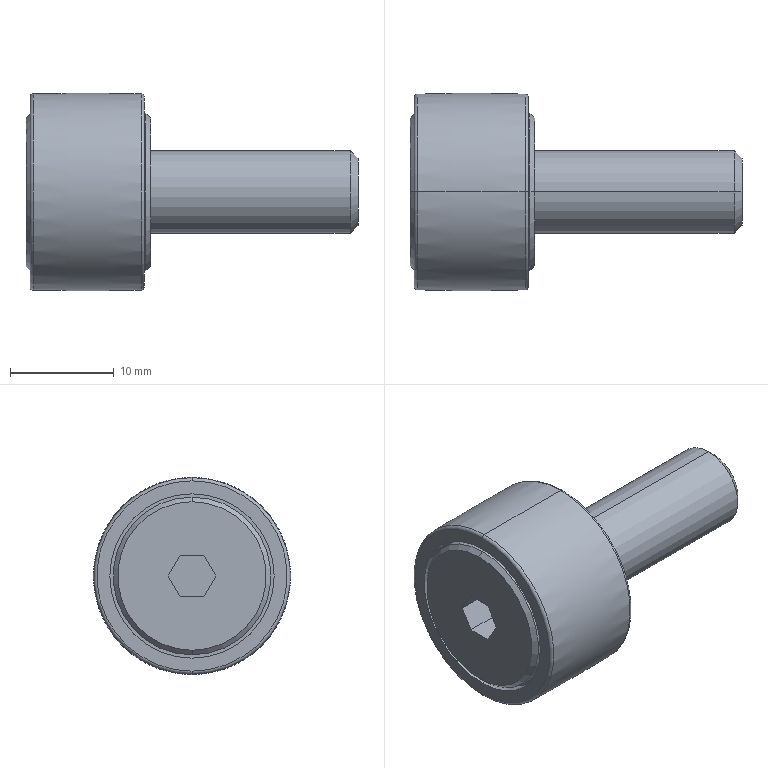Part | STEP file | CF8MUUR-A-1 | 1 solid | 36 faces | box 32 x 19 x 19 mm | volume 4191 mm3 | plane 14 | cylinder 10 | cone 6 | torus 6 | commonest cylinder face diameters 15.2 x4 15.833 x4 8 x2
STEP:
#1=CARTESIAN_POINT('',(32.,0.,-3.233));
#2=VERTEX_POINT('',#1);
#3=CARTESIAN_POINT('',(32.,0.,3.233));
#4=VERTEX_POINT('',#3);
#5=CARTESIAN_POINT('',(32.,0.,0.));
#6=DIRECTION('',(1.,0.,0.));
#7=DIRECTION('',(0.,0.,-1.));
#8=AXIS2_PLACEMENT_3D('',#5,#6,#7);
#9=CIRCLE('',#8,3.233);
#10=EDGE_CURVE('',#2,#4,#9,.T.);
#11=ORIENTED_EDGE('',*,*,#10,.F.);
#12=CARTESIAN_POINT('',(31.233,0.,-4.));
#13=VERTEX_POINT('',#12);
#14=CARTESIAN_POINT('',(31.233,0.,-4.));
#15=DIRECTION('',(-0.7071,0.,-0.7071));
#16=VECTOR('',#15,1000.);
#17=LINE('',#14,#16);
#18=EDGE_CURVE('',#2,#13,#17,.T.);
#19=ORIENTED_EDGE('',*,*,#18,.T.);
#20=CARTESIAN_POINT('',(31.233,0.,4.));
#21=VERTEX_POINT('',#20);
#22=CARTESIAN_POINT('',(31.233,0.,0.));
#23=DIRECTION('',(1.,0.,0.));
#24=DIRECTION('',(0.,0.,-1.));
#25=AXIS2_PLACEMENT_3D('',#22,#23,#24);
#26=CIRCLE('',#25,4.);
#27=EDGE_CURVE('',#13,#21,#26,.T.);
#28=ORIENTED_EDGE('',*,*,#27,.T.);
#29=CARTESIAN_POINT('',(31.233,0.,4.));
#30=DIRECTION('',(-0.7071,0.,0.7071));
#31=VECTOR('',#30,1000.);
#32=LINE('',#29,#31);
#33=EDGE_CURVE('',#4,#21,#32,.T.);
#34=ORIENTED_EDGE('',*,*,#33,.F.);
#35=EDGE_LOOP('',(#11,#19,#28,#34));
#36=FACE_OUTER_BOUND('',#35,.T.);
#37=CARTESIAN_POINT('',(31.233,0.,0.));
#38=DIRECTION('',(-1.,0.,0.));
#39=DIRECTION('',(0.,0.,1.));
#40=AXIS2_PLACEMENT_3D('',#37,#38,#39);
#41=CONICAL_SURFACE('',#40,4.,0.7854);
#42=ADVANCED_FACE('',(#36),#41,.T.);
#43=CARTESIAN_POINT('',(12.,0.,-4.));
#44=VERTEX_POINT('',#43);
#45=CARTESIAN_POINT('',(12.,0.,4.));
#46=VERTEX_POINT('',#45);
#47=CARTESIAN_POINT('',(12.,0.,0.));
#48=DIRECTION('',(1.,0.,0.));
#49=DIRECTION('',(0.,0.,-1.));
#50=AXIS2_PLACEMENT_3D('',#47,#48,#49);
#51=CIRCLE('',#50,4.);
#52=EDGE_CURVE('',#44,#46,#51,.T.);
#53=ORIENTED_EDGE('',*,*,#52,.T.);
#54=CARTESIAN_POINT('',(32.,0.,4.));
#55=DIRECTION('',(1.,0.,0.));
#56=VECTOR('',#55,1000.);
#57=LINE('',#54,#56);
#58=EDGE_CURVE('',#46,#21,#57,.T.);
#59=ORIENTED_EDGE('',*,*,#58,.T.);
#60=ORIENTED_EDGE('',*,*,#27,.F.);
#61=CARTESIAN_POINT('',(32.,0.,-4.));
#62=DIRECTION('',(1.,0.,0.));
#63=VECTOR('',#62,1000.);
#64=LINE('',#61,#63);
#65=EDGE_CURVE('',#44,#13,#64,.T.);
#66=ORIENTED_EDGE('',*,*,#65,.F.);
#67=EDGE_LOOP('',(#53,#59,#60,#66));
#68=FACE_OUTER_BOUND('',#67,.T.);
#69=CARTESIAN_POINT('',(32.,0.,0.));
#70=DIRECTION('',(1.,0.,0.));
#71=DIRECTION('',(0.,0.,-1.));
#72=AXIS2_PLACEMENT_3D('',#69,#70,#71);
#73=CYLINDRICAL_SURFACE('',#72,4.);
#74=ADVANCED_FACE('',(#68),#73,.T.);
#75=CARTESIAN_POINT('',(12.,0.,-7.16));
#76=VERTEX_POINT('',#75);
#77=CARTESIAN_POINT('',(12.,0.,7.16));
#78=VERTEX_POINT('',#77);
#79=CARTESIAN_POINT('',(12.,0.,0.));
#80=DIRECTION('',(1.,0.,0.));
#81=DIRECTION('',(0.,0.,-1.));
#82=AXIS2_PLACEMENT_3D('',#79,#80,#81);
#83=CIRCLE('',#82,7.16);
#84=EDGE_CURVE('',#76,#78,#83,.T.);
#85=ORIENTED_EDGE('',*,*,#84,.F.);
#86=CARTESIAN_POINT('',(11.56,0.,-7.6));
#87=VERTEX_POINT('',#86);
#88=CARTESIAN_POINT('',(11.56,0.,-7.6));
#89=DIRECTION('',(-0.7071,0.,-0.7071));
#90=VECTOR('',#89,1000.);
#91=LINE('',#88,#90);
#92=EDGE_CURVE('',#76,#87,#91,.T.);
#93=ORIENTED_EDGE('',*,*,#92,.T.);
#94=CARTESIAN_POINT('',(11.56,0.,7.6));
#95=VERTEX_POINT('',#94);
#96=CARTESIAN_POINT('',(11.56,0.,0.));
#97=DIRECTION('',(1.,0.,0.));
#98=DIRECTION('',(0.,0.,-1.));
#99=AXIS2_PLACEMENT_3D('',#96,#97,#98);
#100=CIRCLE('',#99,7.6);
#101=EDGE_CURVE('',#87,#95,#100,.T.);
#102=ORIENTED_EDGE('',*,*,#101,.T.);
#103=CARTESIAN_POINT('',(11.56,0.,7.6));
#104=DIRECTION('',(-0.7071,0.,0.7071));
#105=VECTOR('',#104,1000.);
#106=LINE('',#103,#105);
#107=EDGE_CURVE('',#78,#95,#106,.T.);
#108=ORIENTED_EDGE('',*,*,#107,.F.);
#109=EDGE_LOOP('',(#85,#93,#102,#108));
#110=FACE_OUTER_BOUND('',#109,.T.);
#111=CARTESIAN_POINT('',(11.56,0.,0.));
#112=DIRECTION('',(-1.,0.,0.));
#113=DIRECTION('',(0.,0.,1.));
#114=AXIS2_PLACEMENT_3D('',#111,#112,#113);
#115=CONICAL_SURFACE('',#114,7.6,0.7854);
#116=ADVANCED_FACE('',(#110),#115,.T.);
#117=CARTESIAN_POINT('',(10.3,0.,-7.6));
#118=VERTEX_POINT('',#117);
#119=CARTESIAN_POINT('',(10.3,0.,7.6));
#120=VERTEX_POINT('',#119);
#121=CARTESIAN_POINT('',(10.3,0.,0.));
#122=DIRECTION('',(1.,0.,0.));
#123=DIRECTION('',(0.,0.,-1.));
#124=AXIS2_PLACEMENT_3D('',#121,#122,#123);
#125=CIRCLE('',#124,7.6);
#126=EDGE_CURVE('',#118,#120,#125,.T.);
#127=ORIENTED_EDGE('',*,*,#126,.T.);
#128=CARTESIAN_POINT('',(32.,0.,7.6));
#129=DIRECTION('',(1.,0.,0.));
#130=VECTOR('',#129,1000.);
#131=LINE('',#128,#130);
#132=EDGE_CURVE('',#120,#95,#131,.T.);
#133=ORIENTED_EDGE('',*,*,#132,.T.);
#134=ORIENTED_EDGE('',*,*,#101,.F.);
#135=CARTESIAN_POINT('',(32.,0.,-7.6));
#136=DIRECTION('',(1.,0.,0.));
#137=VECTOR('',#136,1000.);
#138=LINE('',#135,#137);
#139=EDGE_CURVE('',#118,#87,#138,.T.);
#140=ORIENTED_EDGE('',*,*,#139,.F.);
#141=EDGE_LOOP('',(#127,#133,#134,#140));
#142=FACE_OUTER_BOUND('',#141,.T.);
#143=CARTESIAN_POINT('',(32.,0.,0.));
#144=DIRECTION('',(1.,0.,0.));
#145=DIRECTION('',(0.,0.,-1.));
#146=AXIS2_PLACEMENT_3D('',#143,#144,#145);
#147=CYLINDRICAL_SURFACE('',#146,7.6);
#148=ADVANCED_FACE('',(#142),#147,.T.);
#149=CARTESIAN_POINT('',(10.3,0.,7.917));
#150=VERTEX_POINT('',#149);
#151=CARTESIAN_POINT('',(10.3,0.,-7.917));
#152=VERTEX_POINT('',#151);
#153=CARTESIAN_POINT('',(10.3,0.,0.));
#154=DIRECTION('',(1.,0.,0.));
#155=DIRECTION('',(0.,0.,-1.));
#156=AXIS2_PLACEMENT_3D('',#153,#154,#155);
#157=CIRCLE('',#156,7.917);
#158=EDGE_CURVE('',#150,#152,#157,.T.);
#159=ORIENTED_EDGE('',*,*,#158,.F.);
#160=CARTESIAN_POINT('',(11.4,0.,7.917));
#161=VERTEX_POINT('',#160);
#162=CARTESIAN_POINT('',(32.,0.,7.917));
#163=DIRECTION('',(1.,0.,0.));
#164=VECTOR('',#163,1000.);
#165=LINE('',#162,#164);
#166=EDGE_CURVE('',#150,#161,#165,.T.);
#167=ORIENTED_EDGE('',*,*,#166,.T.);
#168=CARTESIAN_POINT('',(11.4,0.,-7.917));
#169=VERTEX_POINT('',#168);
#170=CARTESIAN_POINT('',(11.4,0.,0.));
#171=DIRECTION('',(1.,0.,0.));
#172=DIRECTION('',(0.,0.,-1.));
#173=AXIS2_PLACEMENT_3D('',#170,#171,#172);
#174=CIRCLE('',#173,7.917);
#175=EDGE_CURVE('',#161,#169,#174,.T.);
#176=ORIENTED_EDGE('',*,*,#175,.T.);
#177=CARTESIAN_POINT('',(32.,0.,-7.917));
#178=DIRECTION('',(1.,0.,0.));
#179=VECTOR('',#178,1000.);
#180=LINE('',#177,#179);
#181=EDGE_CURVE('',#152,#169,#180,.T.);
#182=ORIENTED_EDGE('',*,*,#181,.F.);
#183=EDGE_LOOP('',(#159,#167,#176,#182));
#184=FACE_OUTER_BOUND('',#183,.T.);
#185=CARTESIAN_POINT('',(32.,0.,0.));
#186=DIRECTION('',(1.,0.,0.));
#187=DIRECTION('',(0.,0.,-1.));
#188=AXIS2_PLACEMENT_3D('',#185,#186,#187);
#189=CYLINDRICAL_SURFACE('',#188,7.917);
#190=ADVANCED_FACE('',(#184),#189,.F.);
#191=CARTESIAN_POINT('',(11.103,0.,-9.474));
#192=VERTEX_POINT('',#191);
#193=CARTESIAN_POINT('',(11.103,0.,9.474));
#194=VERTEX_POINT('',#193);
#195=CARTESIAN_POINT('',(11.103,0.,0.));
#196=DIRECTION('',(1.,0.,0.));
#197=DIRECTION('',(0.,0.,-1.));
#198=AXIS2_PLACEMENT_3D('',#195,#196,#197);
#199=CIRCLE('',#198,9.474);
#200=EDGE_CURVE('',#192,#194,#199,.T.);
#201=ORIENTED_EDGE('',*,*,#200,.T.);
#202=CARTESIAN_POINT('',(11.4,0.,9.174));
#203=VERTEX_POINT('',#202);
#204=CARTESIAN_POINT('',(11.1,0.,9.174));
#205=DIRECTION('',(0.,1.,0.));
#206=DIRECTION('',(0.,0.,1.));
#207=AXIS2_PLACEMENT_3D('',#204,#205,#206);
#208=CIRCLE('',#207,0.3);
#209=EDGE_CURVE('',#194,#203,#208,.T.);
#210=ORIENTED_EDGE('',*,*,#209,.T.);
#211=CARTESIAN_POINT('',(11.4,0.,-9.174));
#212=VERTEX_POINT('',#211);
#213=CARTESIAN_POINT('',(11.4,0.,0.));
#214=DIRECTION('',(1.,0.,0.));
#215=DIRECTION('',(0.,0.,-1.));
#216=AXIS2_PLACEMENT_3D('',#213,#214,#215);
#217=CIRCLE('',#216,9.174);
#218=EDGE_CURVE('',#212,#203,#217,.T.);
#219=ORIENTED_EDGE('',*,*,#218,.F.);
#220=CARTESIAN_POINT('',(11.1,0.,-9.174));
#221=DIRECTION('',(0.,-1.,0.));
#222=DIRECTION('',(1.,0.,0.));
#223=AXIS2_PLACEMENT_3D('',#220,#221,#222);
#224=CIRCLE('',#223,0.3);
#225=EDGE_CURVE('',#192,#212,#224,.T.);
#226=ORIENTED_EDGE('',*,*,#225,.F.);
#227=EDGE_LOOP('',(#201,#210,#219,#226));
#228=FACE_OUTER_BOUND('',#227,.T.);
#229=CARTESIAN_POINT('',(11.1,0.,0.));
#230=DIRECTION('',(1.,0.,0.));
#231=DIRECTION('',(0.,0.,-1.));
#232=AXIS2_PLACEMENT_3D('',#229,#230,#231);
#233=TOROIDAL_SURFACE('',#232,9.174,0.3);
#234=ADVANCED_FACE('',(#228),#233,.T.);
#235=CARTESIAN_POINT('',(0.6968,0.,-9.472));
#236=VERTEX_POINT('',#235);
#237=CARTESIAN_POINT('',(0.6968,0.,9.472));
#238=VERTEX_POINT('',#237);
#239=CARTESIAN_POINT('',(0.6968,0.,0.));
#240=DIRECTION('',(1.,0.,0.));
#241=DIRECTION('',(0.,0.,-1.));
#242=AXIS2_PLACEMENT_3D('',#239,#240,#241);
#243=CIRCLE('',#242,9.472);
#244=EDGE_CURVE('',#236,#238,#243,.T.);
#245=ORIENTED_EDGE('',*,*,#244,.T.);
#246=CARTESIAN_POINT('',(6.,0.,-490.5));
#247=DIRECTION('',(0.,1.,0.));
#248=DIRECTION('',(0.,0.,1.));
#249=AXIS2_PLACEMENT_3D('',#246,#247,#248);
#250=CIRCLE('',#249,500.);
#251=EDGE_CURVE('',#238,#194,#250,.T.);
#252=ORIENTED_EDGE('',*,*,#251,.T.);
#253=ORIENTED_EDGE('',*,*,#200,.F.);
#254=CARTESIAN_POINT('',(6.,0.,490.5));
#255=DIRECTION('',(0.,-1.,0.));
#256=DIRECTION('',(1.,0.,0.));
#257=AXIS2_PLACEMENT_3D('',#254,#255,#256);
#258=CIRCLE('',#257,500.);
#259=EDGE_CURVE('',#236,#192,#258,.T.);
#260=ORIENTED_EDGE('',*,*,#259,.F.);
#261=EDGE_LOOP('',(#245,#252,#253,#260));
#262=FACE_OUTER_BOUND('',#261,.T.);
#263=CARTESIAN_POINT('',(6.,0.,0.));
#264=DIRECTION('',(1.,0.,0.));
#265=DIRECTION('',(0.,0.,-1.));
#266=AXIS2_PLACEMENT_3D('',#263,#264,#265);
#267=TOROIDAL_SURFACE('',#266,-490.5,500.);
#268=ADVANCED_FACE('',(#262),#267,.T.);
#269=CARTESIAN_POINT('',(0.4,0.,-9.172));
#270=VERTEX_POINT('',#269);
#271=CARTESIAN_POINT('',(0.4,0.,9.172));
#272=VERTEX_POINT('',#271);
#273=CARTESIAN_POINT('',(0.4,0.,0.));
#274=DIRECTION('',(1.,0.,0.));
#275=DIRECTION('',(0.,0.,-1.));
#276=AXIS2_PLACEMENT_3D('',#273,#274,#275);
#277=CIRCLE('',#276,9.172);
#278=EDGE_CURVE('',#270,#272,#277,.T.);
#279=ORIENTED_EDGE('',*,*,#278,.T.);
#280=CARTESIAN_POINT('',(0.7,0.,9.172));
#281=DIRECTION('',(0.,1.,0.));
#282=DIRECTION('',(0.,0.,1.));
#283=AXIS2_PLACEMENT_3D('',#280,#281,#282);
#284=CIRCLE('',#283,0.3);
#285=EDGE_CURVE('',#272,#238,#284,.T.);
#286=ORIENTED_EDGE('',*,*,#285,.T.);
#287=ORIENTED_EDGE('',*,*,#244,.F.);
#288=CARTESIAN_POINT('',(0.7,0.,-9.172));
#289=DIRECTION('',(0.,-1.,0.));
#290=DIRECTION('',(1.,0.,0.));
#291=AXIS2_PLACEMENT_3D('',#288,#289,#290);
#292=CIRCLE('',#291,0.3);
#293=EDGE_CURVE('',#270,#236,#292,.T.);
#294=ORIENTED_EDGE('',*,*,#293,.F.);
#295=EDGE_LOOP('',(#279,#286,#287,#294));
#296=FACE_OUTER_BOUND('',#295,.T.);
#297=CARTESIAN_POINT('',(0.7,0.,0.));
#298=DIRECTION('',(1.,0.,0.));
#299=DIRECTION('',(0.,0.,-1.));
#300=AXIS2_PLACEMENT_3D('',#297,#298,#299);
#301=TOROIDAL_SURFACE('',#300,9.172,0.3);
#302=ADVANCED_FACE('',(#296),#301,.T.);
#303=CARTESIAN_POINT('',(0.4,0.,7.917));
#304=VERTEX_POINT('',#303);
#305=CARTESIAN_POINT('',(0.4,0.,-7.917));
#306=VERTEX_POINT('',#305);
#307=CARTESIAN_POINT('',(0.4,0.,0.));
#308=DIRECTION('',(1.,0.,0.));
#309=DIRECTION('',(0.,0.,-1.));
#310=AXIS2_PLACEMENT_3D('',#307,#308,#309);
#311=CIRCLE('',#310,7.917);
#312=EDGE_CURVE('',#304,#306,#311,.T.);
#313=ORIENTED_EDGE('',*,*,#312,.F.);
#314=CARTESIAN_POINT('',(1.5,0.,7.917));
#315=VERTEX_POINT('',#314);
#316=CARTESIAN_POINT('',(32.,0.,7.917));
#317=DIRECTION('',(1.,0.,0.));
#318=VECTOR('',#317,1000.);
#319=LINE('',#316,#318);
#320=EDGE_CURVE('',#304,#315,#319,.T.);
#321=ORIENTED_EDGE('',*,*,#320,.T.);
#322=CARTESIAN_POINT('',(1.5,0.,-7.917));
#323=VERTEX_POINT('',#322);
#324=CARTESIAN_POINT('',(1.5,0.,0.));
#325=DIRECTION('',(1.,0.,0.));
#326=DIRECTION('',(0.,0.,-1.));
#327=AXIS2_PLACEMENT_3D('',#324,#325,#326);
#328=CIRCLE('',#327,7.917);
#329=EDGE_CURVE('',#315,#323,#328,.T.);
#330=ORIENTED_EDGE('',*,*,#329,.T.);
#331=CARTESIAN_POINT('',(32.,0.,-7.917));
#332=DIRECTION('',(1.,0.,0.));
#333=VECTOR('',#332,1000.);
#334=LINE('',#331,#333);
#335=EDGE_CURVE('',#306,#323,#334,.T.);
#336=ORIENTED_EDGE('',*,*,#335,.F.);
#337=EDGE_LOOP('',(#313,#321,#330,#336));
#338=FACE_OUTER_BOUND('',#337,.T.);
#339=CARTESIAN_POINT('',(32.,0.,0.));
#340=DIRECTION('',(1.,0.,0.));
#341=DIRECTION('',(0.,0.,-1.));
#342=AXIS2_PLACEMENT_3D('',#339,#340,#341);
#343=CYLINDRICAL_SURFACE('',#342,7.917);
#344=ADVANCED_FACE('',(#338),#343,.F.);
#345=CARTESIAN_POINT('',(0.44,0.,-7.6));
#346=VERTEX_POINT('',#345);
#347=CARTESIAN_POINT('',(0.44,0.,7.6));
#348=VERTEX_POINT('',#347);
#349=CARTESIAN_POINT('',(0.44,0.,0.));
#350=DIRECTION('',(1.,0.,0.));
#351=DIRECTION('',(0.,0.,-1.));
#352=AXIS2_PLACEMENT_3D('',#349,#350,#351);
#353=CIRCLE('',#352,7.6);
#354=EDGE_CURVE('',#346,#348,#353,.T.);
#355=ORIENTED_EDGE('',*,*,#354,.T.);
#356=CARTESIAN_POINT('',(1.5,0.,7.6));
#357=VERTEX_POINT('',#356);
#358=CARTESIAN_POINT('',(32.,0.,7.6));
#359=DIRECTION('',(1.,0.,0.));
#360=VECTOR('',#359,1000.);
#361=LINE('',#358,#360);
#362=EDGE_CURVE('',#348,#357,#361,.T.);
#363=ORIENTED_EDGE('',*,*,#362,.T.);
#364=CARTESIAN_POINT('',(1.5,0.,-7.6));
#365=VERTEX_POINT('',#364);
#366=CARTESIAN_POINT('',(1.5,0.,0.));
#367=DIRECTION('',(1.,0.,0.));
#368=DIRECTION('',(0.,0.,-1.));
#369=AXIS2_PLACEMENT_3D('',#366,#367,#368);
#370=CIRCLE('',#369,7.6);
#371=EDGE_CURVE('',#365,#357,#370,.T.);
#372=ORIENTED_EDGE('',*,*,#371,.F.);
#373=CARTESIAN_POINT('',(32.,0.,-7.6));
#374=DIRECTION('',(1.,0.,0.));
#375=VECTOR('',#374,1000.);
#376=LINE('',#373,#375);
#377=EDGE_CURVE('',#346,#365,#376,.T.);
#378=ORIENTED_EDGE('',*,*,#377,.F.);
#379=EDGE_LOOP('',(#355,#363,#372,#378));
#380=FACE_OUTER_BOUND('',#379,.T.);
#381=CARTESIAN_POINT('',(32.,0.,0.));
#382=DIRECTION('',(1.,0.,0.));
#383=DIRECTION('',(0.,0.,-1.));
#384=AXIS2_PLACEMENT_3D('',#381,#382,#383);
#385=CYLINDRICAL_SURFACE('',#384,7.6);
#386=ADVANCED_FACE('',(#380),#385,.T.);
#387=CARTESIAN_POINT('',(0.,0.,-7.16));
#388=VERTEX_POINT('',#387);
#389=CARTESIAN_POINT('',(0.,0.,7.16));
#390=VERTEX_POINT('',#389);
#391=CARTESIAN_POINT('',(0.,0.,0.));
#392=DIRECTION('',(1.,0.,0.));
#393=DIRECTION('',(0.,0.,-1.));
#394=AXIS2_PLACEMENT_3D('',#391,#392,#393);
#395=CIRCLE('',#394,7.16);
#396=EDGE_CURVE('',#388,#390,#395,.T.);
#397=ORIENTED_EDGE('',*,*,#396,.T.);
#398=CARTESIAN_POINT('',(0.,0.,7.16));
#399=DIRECTION('',(0.7071,0.,0.7071));
#400=VECTOR('',#399,1000.);
#401=LINE('',#398,#400);
#402=EDGE_CURVE('',#390,#348,#401,.T.);
#403=ORIENTED_EDGE('',*,*,#402,.T.);
#404=ORIENTED_EDGE('',*,*,#354,.F.);
#405=CARTESIAN_POINT('',(0.,0.,-7.16));
#406=DIRECTION('',(0.7071,0.,-0.7071));
#407=VECTOR('',#406,1000.);
#408=LINE('',#405,#407);
#409=EDGE_CURVE('',#388,#346,#408,.T.);
#410=ORIENTED_EDGE('',*,*,#409,.F.);
#411=EDGE_LOOP('',(#397,#403,#404,#410));
#412=FACE_OUTER_BOUND('',#411,.T.);
#413=CARTESIAN_POINT('',(0.,0.,0.));
#414=DIRECTION('',(1.,0.,0.));
#415=DIRECTION('',(0.,0.,-1.));
#416=AXIS2_PLACEMENT_3D('',#413,#414,#415);
#417=CONICAL_SURFACE('',#416,7.16,0.7854);
#418=ADVANCED_FACE('',(#412),#417,.T.);
#419=ORIENTED_EDGE('',*,*,#396,.F.);
#420=CARTESIAN_POINT('',(0.,0.,0.));
#421=DIRECTION('',(1.,0.,0.));
#422=DIRECTION('',(0.,0.,-1.));
#423=AXIS2_PLACEMENT_3D('',#420,#421,#422);
#424=CIRCLE('',#423,7.16);
#425=EDGE_CURVE('',#390,#388,#424,.T.);
#426=ORIENTED_EDGE('',*,*,#425,.F.);
#427=EDGE_LOOP('',(#419,#426));
#428=FACE_OUTER_BOUND('',#427,.T.);
#429=CARTESIAN_POINT('',(0.,1.155,2.));
#430=VERTEX_POINT('',#429);
#431=CARTESIAN_POINT('',(0.,-1.155,2.));
#432=VERTEX_POINT('',#431);
#433=CARTESIAN_POINT('',(0.,1.155,2.));
#434=DIRECTION('',(0.,-1.,0.));
#435=VECTOR('',#434,1000.);
#436=LINE('',#433,#435);
#437=EDGE_CURVE('',#430,#432,#436,.T.);
#438=ORIENTED_EDGE('',*,*,#437,.T.);
#439=CARTESIAN_POINT('',(0.,-2.309,0.));
#440=VERTEX_POINT('',#439);
#441=CARTESIAN_POINT('',(0.,-1.155,2.));
#442=DIRECTION('',(0.,-0.5,-0.866));
#443=VECTOR('',#442,1000.);
#444=LINE('',#441,#443);
#445=EDGE_CURVE('',#432,#440,#444,.T.);
#446=ORIENTED_EDGE('',*,*,#445,.T.);
#447=CARTESIAN_POINT('',(0.,-1.155,-2.));
#448=VERTEX_POINT('',#447);
#449=CARTESIAN_POINT('',(0.,-2.309,0.));
#450=DIRECTION('',(0.,0.5,-0.866));
#451=VECTOR('',#450,1000.);
#452=LINE('',#449,#451);
#453=EDGE_CURVE('',#440,#448,#452,.T.);
#454=ORIENTED_EDGE('',*,*,#453,.T.);
#455=CARTESIAN_POINT('',(0.,1.155,-2.));
#456=VERTEX_POINT('',#455);
#457=CARTESIAN_POINT('',(0.,-1.155,-2.));
#458=DIRECTION('',(0.,1.,0.));
#459=VECTOR('',#458,1000.);
#460=LINE('',#457,#459);
#461=EDGE_CURVE('',#448,#456,#460,.T.);
#462=ORIENTED_EDGE('',*,*,#461,.T.);
#463=CARTESIAN_POINT('',(0.,2.309,0.));
#464=VERTEX_POINT('',#463);
#465=CARTESIAN_POINT('',(0.,1.155,-2.));
#466=DIRECTION('',(0.,0.5,0.866));
#467=VECTOR('',#466,1000.);
#468=LINE('',#465,#467);
#469=EDGE_CURVE('',#456,#464,#468,.T.);
#470=ORIENTED_EDGE('',*,*,#469,.T.);
#471=CARTESIAN_POINT('',(0.,2.309,0.));
#472=DIRECTION('',(0.,-0.5,0.866));
#473=VECTOR('',#472,1000.);
#474=LINE('',#471,#473);
#475=EDGE_CURVE('',#464,#430,#474,.T.);
#476=ORIENTED_EDGE('',*,*,#475,.T.);
#477=EDGE_LOOP('',(#438,#446,#454,#462,#470,#476));
#478=FACE_BOUND('',#477,.T.);
#479=CARTESIAN_POINT('',(0.,0.,0.));
#480=DIRECTION('',(1.,0.,0.));
#481=DIRECTION('',(0.,0.,-1.));
#482=AXIS2_PLACEMENT_3D('',#479,#480,#481);
#483=PLANE('',#482);
#484=ADVANCED_FACE('',(#428,#478),#483,.F.);
#485=ORIENTED_EDGE('',*,*,#402,.F.);
#486=ORIENTED_EDGE('',*,*,#425,.T.);
#487=ORIENTED_EDGE('',*,*,#409,.T.);
#488=CARTESIAN_POINT('',(0.44,0.,0.));
#489=DIRECTION('',(1.,0.,0.));
#490=DIRECTION('',(0.,0.,-1.));
#491=AXIS2_PLACEMENT_3D('',#488,#489,#490);
#492=CIRCLE('',#491,7.6);
#493=EDGE_CURVE('',#348,#346,#492,.T.);
#494=ORIENTED_EDGE('',*,*,#493,.F.);
#495=EDGE_LOOP('',(#485,#486,#487,#494));
#496=FACE_OUTER_BOUND('',#495,.T.);
#497=CARTESIAN_POINT('',(0.,0.,0.));
#498=DIRECTION('',(1.,0.,0.));
#499=DIRECTION('',(0.,0.,-1.));
#500=AXIS2_PLACEMENT_3D('',#497,#498,#499);
#501=CONICAL_SURFACE('',#500,7.16,0.7854);
#502=ADVANCED_FACE('',(#496),#501,.T.);
#503=ORIENTED_EDGE('',*,*,#362,.F.);
#504=ORIENTED_EDGE('',*,*,#493,.T.);
#505=ORIENTED_EDGE('',*,*,#377,.T.);
#506=CARTESIAN_POINT('',(1.5,0.,0.));
#507=DIRECTION('',(1.,0.,0.));
#508=DIRECTION('',(0.,0.,-1.));
#509=AXIS2_PLACEMENT_3D('',#506,#507,#508);
#510=CIRCLE('',#509,7.6);
#511=EDGE_CURVE('',#357,#365,#510,.T.);
#512=ORIENTED_EDGE('',*,*,#511,.F.);
#513=EDGE_LOOP('',(#503,#504,#505,#512));
#514=FACE_OUTER_BOUND('',#513,.T.);
#515=CARTESIAN_POINT('',(32.,0.,0.));
#516=DIRECTION('',(1.,0.,0.));
#517=DIRECTION('',(0.,0.,-1.));
#518=AXIS2_PLACEMENT_3D('',#515,#516,#517);
#519=CYLINDRICAL_SURFACE('',#518,7.6);
#520=ADVANCED_FACE('',(#514),#519,.T.);
#521=CARTESIAN_POINT('',(1.5,0.,0.));
#522=DIRECTION('',(1.,0.,0.));
#523=DIRECTION('',(0.,0.,-1.));
#524=AXIS2_PLACEMENT_3D('',#521,#522,#523);
#525=CIRCLE('',#524,7.917);
#526=EDGE_CURVE('',#323,#315,#525,.T.);
#527=ORIENTED_EDGE('',*,*,#526,.F.);
#528=ORIENTED_EDGE('',*,*,#329,.F.);
#529=EDGE_LOOP('',(#527,#528));
#530=FACE_OUTER_BOUND('',#529,.T.);
#531=ORIENTED_EDGE('',*,*,#371,.T.);
#532=ORIENTED_EDGE('',*,*,#511,.T.);
#533=EDGE_LOOP('',(#531,#532));
#534=FACE_BOUND('',#533,.T.);
#535=CARTESIAN_POINT('',(1.5,7.6,0.));
#536=DIRECTION('',(1.,0.,0.));
#537=DIRECTION('',(0.,0.,-1.));
#538=AXIS2_PLACEMENT_3D('',#535,#536,#537);
#539=PLANE('',#538);
#540=ADVANCED_FACE('',(#530,#534),#539,.F.);
#541=ORIENTED_EDGE('',*,*,#320,.F.);
#542=CARTESIAN_POINT('',(0.4,0.,0.));
#543=DIRECTION('',(1.,0.,0.));
#544=DIRECTION('',(0.,0.,-1.));
#545=AXIS2_PLACEMENT_3D('',#542,#543,#544);
#546=CIRCLE('',#545,7.917);
#547=EDGE_CURVE('',#306,#304,#546,.T.);
#548=ORIENTED_EDGE('',*,*,#547,.F.);
#549=ORIENTED_EDGE('',*,*,#335,.T.);
#550=ORIENTED_EDGE('',*,*,#526,.T.);
#551=EDGE_LOOP('',(#541,#548,#549,#550));
#552=FACE_OUTER_BOUND('',#551,.T.);
#553=CARTESIAN_POINT('',(32.,0.,0.));
#554=DIRECTION('',(1.,0.,0.));
#555=DIRECTION('',(0.,0.,-1.));
#556=AXIS2_PLACEMENT_3D('',#553,#554,#555);
#557=CYLINDRICAL_SURFACE('',#556,7.917);
#558=ADVANCED_FACE('',(#552),#557,.F.);
#559=ORIENTED_EDGE('',*,*,#278,.F.);
#560=CARTESIAN_POINT('',(0.4,0.,0.));
#561=DIRECTION('',(1.,0.,0.));
#562=DIRECTION('',(0.,0.,-1.));
#563=AXIS2_PLACEMENT_3D('',#560,#561,#562);
#564=CIRCLE('',#563,9.172);
#565=EDGE_CURVE('',#272,#270,#564,.T.);
#566=ORIENTED_EDGE('',*,*,#565,.F.);
#567=EDGE_LOOP('',(#559,#566));
#568=FACE_OUTER_BOUND('',#567,.T.);
#569=ORIENTED_EDGE('',*,*,#547,.T.);
#570=ORIENTED_EDGE('',*,*,#312,.T.);
#571=EDGE_LOOP('',(#569,#570));
#572=FACE_BOUND('',#571,.T.);
#573=CARTESIAN_POINT('',(0.4,7.917,0.));
#574=DIRECTION('',(1.,0.,0.));
#575=DIRECTION('',(0.,0.,-1.));
#576=AXIS2_PLACEMENT_3D('',#573,#574,#575);
#577=PLANE('',#576);
#578=ADVANCED_FACE('',(#568,#572),#577,.F.);
#579=ORIENTED_EDGE('',*,*,#285,.F.);
#580=ORIENTED_EDGE('',*,*,#565,.T.);
#581=ORIENTED_EDGE('',*,*,#293,.T.);
#582=CARTESIAN_POINT('',(0.6968,0.,0.));
#583=DIRECTION('',(1.,0.,0.));
#584=DIRECTION('',(0.,0.,-1.));
#585=AXIS2_PLACEMENT_3D('',#582,#583,#584);
#586=CIRCLE('',#585,9.472);
#587=EDGE_CURVE('',#238,#236,#586,.T.);
#588=ORIENTED_EDGE('',*,*,#587,.F.);
#589=EDGE_LOOP('',(#579,#580,#581,#588));
#590=FACE_OUTER_BOUND('',#589,.T.);
#591=CARTESIAN_POINT('',(0.7,0.,0.));
#592=DIRECTION('',(1.,0.,0.));
#593=DIRECTION('',(0.,0.,-1.));
#594=AXIS2_PLACEMENT_3D('',#591,#592,#593);
#595=TOROIDAL_SURFACE('',#594,9.172,0.3);
#596=ADVANCED_FACE('',(#590),#595,.T.);
#597=ORIENTED_EDGE('',*,*,#251,.F.);
#598=ORIENTED_EDGE('',*,*,#587,.T.);
#599=ORIENTED_EDGE('',*,*,#259,.T.);
#600=CARTESIAN_POINT('',(11.103,0.,0.));
#601=DIRECTION('',(1.,0.,0.));
#602=DIRECTION('',(0.,0.,-1.));
#603=AXIS2_PLACEMENT_3D('',#600,#601,#602);
#604=CIRCLE('',#603,9.474);
#605=EDGE_CURVE('',#194,#192,#604,.T.);
#606=ORIENTED_EDGE('',*,*,#605,.F.);
#607=EDGE_LOOP('',(#597,#598,#599,#606));
#608=FACE_OUTER_BOUND('',#607,.T.);
#609=CARTESIAN_POINT('',(6.,0.,0.));
#610=DIRECTION('',(1.,0.,0.));
#611=DIRECTION('',(0.,0.,-1.));
#612=AXIS2_PLACEMENT_3D('',#609,#610,#611);
#613=TOROIDAL_SURFACE('',#612,-490.5,500.);
#614=ADVANCED_FACE('',(#608),#613,.T.);
#615=ORIENTED_EDGE('',*,*,#209,.F.);
#616=ORIENTED_EDGE('',*,*,#605,.T.);
#617=ORIENTED_EDGE('',*,*,#225,.T.);
#618=CARTESIAN_POINT('',(11.4,0.,0.));
#619=DIRECTION('',(1.,0.,0.));
#620=DIRECTION('',(0.,0.,-1.));
#621=AXIS2_PLACEMENT_3D('',#618,#619,#620);
#622=CIRCLE('',#621,9.174);
#623=EDGE_CURVE('',#203,#212,#622,.T.);
#624=ORIENTED_EDGE('',*,*,#623,.F.);
#625=EDGE_LOOP('',(#615,#616,#617,#624));
#626=FACE_OUTER_BOUND('',#625,.T.);
#627=CARTESIAN_POINT('',(11.1,0.,0.));
#628=DIRECTION('',(1.,0.,0.));
#629=DIRECTION('',(0.,0.,-1.));
#630=AXIS2_PLACEMENT_3D('',#627,#628,#629);
#631=TOROIDAL_SURFACE('',#630,9.174,0.3);
#632=ADVANCED_FACE('',(#626),#631,.T.);
#633=CARTESIAN_POINT('',(11.4,0.,0.));
#634=DIRECTION('',(1.,0.,0.));
#635=DIRECTION('',(0.,0.,-1.));
#636=AXIS2_PLACEMENT_3D('',#633,#634,#635);
#637=CIRCLE('',#636,7.917);
#638=EDGE_CURVE('',#169,#161,#637,.T.);
#639=ORIENTED_EDGE('',*,*,#638,.F.);
#640=ORIENTED_EDGE('',*,*,#175,.F.);
#641=EDGE_LOOP('',(#639,#640));
#642=FACE_BOUND('',#641,.T.);
#643=ORIENTED_EDGE('',*,*,#218,.T.);
#644=ORIENTED_EDGE('',*,*,#623,.T.);
#645=EDGE_LOOP('',(#643,#644));
#646=FACE_OUTER_BOUND('',#645,.T.);
#647=CARTESIAN_POINT('',(11.4,9.174,0.));
#648=DIRECTION('',(-1.,0.,0.));
#649=DIRECTION('',(0.,0.,1.));
#650=AXIS2_PLACEMENT_3D('',#647,#648,#649);
#651=PLANE('',#650);
#652=ADVANCED_FACE('',(#642,#646),#651,.F.);
#653=ORIENTED_EDGE('',*,*,#166,.F.);
#654=CARTESIAN_POINT('',(10.3,0.,0.));
#655=DIRECTION('',(1.,0.,0.));
#656=DIRECTION('',(0.,0.,-1.));
#657=AXIS2_PLACEMENT_3D('',#654,#655,#656);
#658=CIRCLE('',#657,7.917);
#659=EDGE_CURVE('',#152,#150,#658,.T.);
#660=ORIENTED_EDGE('',*,*,#659,.F.);
#661=ORIENTED_EDGE('',*,*,#181,.T.);
#662=ORIENTED_EDGE('',*,*,#638,.T.);
#663=EDGE_LOOP('',(#653,#660,#661,#662));
#664=FACE_OUTER_BOUND('',#663,.T.);
#665=CARTESIAN_POINT('',(32.,0.,0.));
#666=DIRECTION('',(1.,0.,0.));
#667=DIRECTION('',(0.,0.,-1.));
#668=AXIS2_PLACEMENT_3D('',#665,#666,#667);
#669=CYLINDRICAL_SURFACE('',#668,7.917);
#670=ADVANCED_FACE('',(#664),#669,.F.);
#671=ORIENTED_EDGE('',*,*,#126,.F.);
#672=CARTESIAN_POINT('',(10.3,0.,0.));
#673=DIRECTION('',(1.,0.,0.));
#674=DIRECTION('',(0.,0.,-1.));
#675=AXIS2_PLACEMENT_3D('',#672,#673,#674);
#676=CIRCLE('',#675,7.6);
#677=EDGE_CURVE('',#120,#118,#676,.T.);
#678=ORIENTED_EDGE('',*,*,#677,.F.);
#679=EDGE_LOOP('',(#671,#678));
#680=FACE_BOUND('',#679,.T.);
#681=ORIENTED_EDGE('',*,*,#659,.T.);
#682=ORIENTED_EDGE('',*,*,#158,.T.);
#683=EDGE_LOOP('',(#681,#682));
#684=FACE_OUTER_BOUND('',#683,.T.);
#685=CARTESIAN_POINT('',(10.3,7.917,0.));
#686=DIRECTION('',(-1.,0.,0.));
#687=DIRECTION('',(0.,0.,1.));
#688=AXIS2_PLACEMENT_3D('',#685,#686,#687);
#689=PLANE('',#688);
#690=ADVANCED_FACE('',(#680,#684),#689,.F.);
#691=ORIENTED_EDGE('',*,*,#132,.F.);
#692=ORIENTED_EDGE('',*,*,#677,.T.);
#693=ORIENTED_EDGE('',*,*,#139,.T.);
#694=CARTESIAN_POINT('',(11.56,0.,0.));
#695=DIRECTION('',(1.,0.,0.));
#696=DIRECTION('',(0.,0.,-1.));
#697=AXIS2_PLACEMENT_3D('',#694,#695,#696);
#698=CIRCLE('',#697,7.6);
#699=EDGE_CURVE('',#95,#87,#698,.T.);
#700=ORIENTED_EDGE('',*,*,#699,.F.);
#701=EDGE_LOOP('',(#691,#692,#693,#700));
#702=FACE_OUTER_BOUND('',#701,.T.);
#703=CARTESIAN_POINT('',(32.,0.,0.));
#704=DIRECTION('',(1.,0.,0.));
#705=DIRECTION('',(0.,0.,-1.));
#706=AXIS2_PLACEMENT_3D('',#703,#704,#705);
#707=CYLINDRICAL_SURFACE('',#706,7.6);
#708=ADVANCED_FACE('',(#702),#707,.T.);
#709=ORIENTED_EDGE('',*,*,#92,.F.);
#710=CARTESIAN_POINT('',(12.,0.,0.));
#711=DIRECTION('',(1.,0.,0.));
#712=DIRECTION('',(0.,0.,-1.));
#713=AXIS2_PLACEMENT_3D('',#710,#711,#712);
#714=CIRCLE('',#713,7.16);
#715=EDGE_CURVE('',#78,#76,#714,.T.);
#716=ORIENTED_EDGE('',*,*,#715,.F.);
#717=ORIENTED_EDGE('',*,*,#107,.T.);
#718=ORIENTED_EDGE('',*,*,#699,.T.);
#719=EDGE_LOOP('',(#709,#716,#717,#718));
#720=FACE_OUTER_BOUND('',#719,.T.);
#721=CARTESIAN_POINT('',(11.56,0.,0.));
#722=DIRECTION('',(-1.,0.,0.));
#723=DIRECTION('',(0.,0.,1.));
#724=AXIS2_PLACEMENT_3D('',#721,#722,#723);
#725=CONICAL_SURFACE('',#724,7.6,0.7854);
#726=ADVANCED_FACE('',(#720),#725,.T.);
#727=ORIENTED_EDGE('',*,*,#52,.F.);
#728=CARTESIAN_POINT('',(12.,0.,0.));
#729=DIRECTION('',(1.,0.,0.));
#730=DIRECTION('',(0.,0.,-1.));
#731=AXIS2_PLACEMENT_3D('',#728,#729,#730);
#732=CIRCLE('',#731,4.);
#733=EDGE_CURVE('',#46,#44,#732,.T.);
#734=ORIENTED_EDGE('',*,*,#733,.F.);
#735=EDGE_LOOP('',(#727,#734));
#736=FACE_BOUND('',#735,.T.);
#737=ORIENTED_EDGE('',*,*,#715,.T.);
#738=ORIENTED_EDGE('',*,*,#84,.T.);
#739=EDGE_LOOP('',(#737,#738));
#740=FACE_OUTER_BOUND('',#739,.T.);
#741=CARTESIAN_POINT('',(12.,7.16,0.));
#742=DIRECTION('',(-1.,0.,0.));
#743=DIRECTION('',(0.,0.,1.));
#744=AXIS2_PLACEMENT_3D('',#741,#742,#743);
#745=PLANE('',#744);
#746=ADVANCED_FACE('',(#736,#740),#745,.F.);
#747=ORIENTED_EDGE('',*,*,#58,.F.);
#748=ORIENTED_EDGE('',*,*,#733,.T.);
#749=ORIENTED_EDGE('',*,*,#65,.T.);
#750=CARTESIAN_POINT('',(31.233,0.,0.));
#751=DIRECTION('',(1.,0.,0.));
#752=DIRECTION('',(0.,0.,-1.));
#753=AXIS2_PLACEMENT_3D('',#750,#751,#752);
#754=CIRCLE('',#753,4.);
#755=EDGE_CURVE('',#21,#13,#754,.T.);
#756=ORIENTED_EDGE('',*,*,#755,.F.);
#757=EDGE_LOOP('',(#747,#748,#749,#756));
#758=FACE_OUTER_BOUND('',#757,.T.);
#759=CARTESIAN_POINT('',(32.,0.,0.));
#760=DIRECTION('',(1.,0.,0.));
#761=DIRECTION('',(0.,0.,-1.));
#762=AXIS2_PLACEMENT_3D('',#759,#760,#761);
#763=CYLINDRICAL_SURFACE('',#762,4.);
#764=ADVANCED_FACE('',(#758),#763,.T.);
#765=ORIENTED_EDGE('',*,*,#18,.F.);
#766=CARTESIAN_POINT('',(32.,0.,0.));
#767=DIRECTION('',(1.,0.,0.));
#768=DIRECTION('',(0.,0.,-1.));
#769=AXIS2_PLACEMENT_3D('',#766,#767,#768);
#770=CIRCLE('',#769,3.233);
#771=EDGE_CURVE('',#4,#2,#770,.T.);
#772=ORIENTED_EDGE('',*,*,#771,.F.);
#773=ORIENTED_EDGE('',*,*,#33,.T.);
#774=ORIENTED_EDGE('',*,*,#755,.T.);
#775=EDGE_LOOP('',(#765,#772,#773,#774));
#776=FACE_OUTER_BOUND('',#775,.T.);
#777=CARTESIAN_POINT('',(31.233,0.,0.));
#778=DIRECTION('',(-1.,0.,0.));
#779=DIRECTION('',(0.,0.,1.));
#780=AXIS2_PLACEMENT_3D('',#777,#778,#779);
#781=CONICAL_SURFACE('',#780,4.,0.7854);
#782=ADVANCED_FACE('',(#776),#781,.T.);
#783=ORIENTED_EDGE('',*,*,#771,.T.);
#784=ORIENTED_EDGE('',*,*,#10,.T.);
#785=EDGE_LOOP('',(#783,#784));
#786=FACE_OUTER_BOUND('',#785,.T.);
#787=CARTESIAN_POINT('',(32.,3.233,0.));
#788=DIRECTION('',(-1.,0.,0.));
#789=DIRECTION('',(0.,0.,1.));
#790=AXIS2_PLACEMENT_3D('',#787,#788,#789);
#791=PLANE('',#790);
#792=ADVANCED_FACE('',(#786),#791,.F.);
#793=ORIENTED_EDGE('',*,*,#437,.F.);
#794=CARTESIAN_POINT('',(4.,1.155,2.));
#795=VERTEX_POINT('',#794);
#796=CARTESIAN_POINT('',(4.,1.155,2.));
#797=DIRECTION('',(-1.,0.,0.));
#798=VECTOR('',#797,1000.);
#799=LINE('',#796,#798);
#800=EDGE_CURVE('',#795,#430,#799,.T.);
#801=ORIENTED_EDGE('',*,*,#800,.F.);
#802=CARTESIAN_POINT('',(4.,-1.155,2.));
#803=VERTEX_POINT('',#802);
#804=CARTESIAN_POINT('',(4.,1.155,2.));
#805=DIRECTION('',(0.,-1.,0.));
#806=VECTOR('',#805,1000.);
#807=LINE('',#804,#806);
#808=EDGE_CURVE('',#795,#803,#807,.T.);
#809=ORIENTED_EDGE('',*,*,#808,.T.);
#810=CARTESIAN_POINT('',(4.,-1.155,2.));
#811=DIRECTION('',(-1.,0.,0.));
#812=VECTOR('',#811,1000.);
#813=LINE('',#810,#812);
#814=EDGE_CURVE('',#803,#432,#813,.T.);
#815=ORIENTED_EDGE('',*,*,#814,.T.);
#816=EDGE_LOOP('',(#793,#801,#809,#815));
#817=FACE_OUTER_BOUND('',#816,.T.);
#818=CARTESIAN_POINT('',(4.,1.155,2.));
#819=DIRECTION('',(0.,0.,-1.));
#820=DIRECTION('',(-1.,0.,0.));
#821=AXIS2_PLACEMENT_3D('',#818,#819,#820);
#822=PLANE('',#821);
#823=ADVANCED_FACE('',(#817),#822,.T.);
#824=ORIENTED_EDGE('',*,*,#445,.F.);
#825=ORIENTED_EDGE('',*,*,#814,.F.);
#826=CARTESIAN_POINT('',(4.,-2.309,0.));
#827=VERTEX_POINT('',#826);
#828=CARTESIAN_POINT('',(4.,-1.155,2.));
#829=DIRECTION('',(0.,-0.5,-0.866));
#830=VECTOR('',#829,1000.);
#831=LINE('',#828,#830);
#832=EDGE_CURVE('',#803,#827,#831,.T.);
#833=ORIENTED_EDGE('',*,*,#832,.T.);
#834=CARTESIAN_POINT('',(4.,-2.309,0.));
#835=DIRECTION('',(-1.,0.,0.));
#836=VECTOR('',#835,1000.);
#837=LINE('',#834,#836);
#838=EDGE_CURVE('',#827,#440,#837,.T.);
#839=ORIENTED_EDGE('',*,*,#838,.T.);
#840=EDGE_LOOP('',(#824,#825,#833,#839));
#841=FACE_OUTER_BOUND('',#840,.T.);
#842=CARTESIAN_POINT('',(4.,-1.155,2.));
#843=DIRECTION('',(0.,0.866,-0.5));
#844=DIRECTION('',(0.,0.5,0.866));
#845=AXIS2_PLACEMENT_3D('',#842,#843,#844);
#846=PLANE('',#845);
#847=ADVANCED_FACE('',(#841),#846,.T.);
#848=ORIENTED_EDGE('',*,*,#453,.F.);
#849=ORIENTED_EDGE('',*,*,#838,.F.);
#850=CARTESIAN_POINT('',(4.,-1.155,-2.));
#851=VERTEX_POINT('',#850);
#852=CARTESIAN_POINT('',(4.,-2.309,0.));
#853=DIRECTION('',(0.,0.5,-0.866));
#854=VECTOR('',#853,1000.);
#855=LINE('',#852,#854);
#856=EDGE_CURVE('',#827,#851,#855,.T.);
#857=ORIENTED_EDGE('',*,*,#856,.T.);
#858=CARTESIAN_POINT('',(4.,-1.155,-2.));
#859=DIRECTION('',(-1.,0.,0.));
#860=VECTOR('',#859,1000.);
#861=LINE('',#858,#860);
#862=EDGE_CURVE('',#851,#448,#861,.T.);
#863=ORIENTED_EDGE('',*,*,#862,.T.);
#864=EDGE_LOOP('',(#848,#849,#857,#863));
#865=FACE_OUTER_BOUND('',#864,.T.);
#866=CARTESIAN_POINT('',(4.,-2.309,0.));
#867=DIRECTION('',(0.,0.866,0.5));
#868=DIRECTION('',(0.,-0.5,0.866));
#869=AXIS2_PLACEMENT_3D('',#866,#867,#868);
#870=PLANE('',#869);
#871=ADVANCED_FACE('',(#865),#870,.T.);
#872=ORIENTED_EDGE('',*,*,#461,.F.);
#873=ORIENTED_EDGE('',*,*,#862,.F.);
#874=CARTESIAN_POINT('',(4.,1.155,-2.));
#875=VERTEX_POINT('',#874);
#876=CARTESIAN_POINT('',(4.,-1.155,-2.));
#877=DIRECTION('',(0.,1.,0.));
#878=VECTOR('',#877,1000.);
#879=LINE('',#876,#878);
#880=EDGE_CURVE('',#851,#875,#879,.T.);
#881=ORIENTED_EDGE('',*,*,#880,.T.);
#882=CARTESIAN_POINT('',(4.,1.155,-2.));
#883=DIRECTION('',(-1.,0.,0.));
#884=VECTOR('',#883,1000.);
#885=LINE('',#882,#884);
#886=EDGE_CURVE('',#875,#456,#885,.T.);
#887=ORIENTED_EDGE('',*,*,#886,.T.);
#888=EDGE_LOOP('',(#872,#873,#881,#887));
#889=FACE_OUTER_BOUND('',#888,.T.);
#890=CARTESIAN_POINT('',(4.,-1.155,-2.));
#891=DIRECTION('',(0.,0.,1.));
#892=DIRECTION('',(1.,0.,0.));
#893=AXIS2_PLACEMENT_3D('',#890,#891,#892);
#894=PLANE('',#893);
#895=ADVANCED_FACE('',(#889),#894,.T.);
#896=ORIENTED_EDGE('',*,*,#469,.F.);
#897=ORIENTED_EDGE('',*,*,#886,.F.);
#898=CARTESIAN_POINT('',(4.,2.309,0.));
#899=VERTEX_POINT('',#898);
#900=CARTESIAN_POINT('',(4.,1.155,-2.));
#901=DIRECTION('',(0.,0.5,0.866));
#902=VECTOR('',#901,1000.);
#903=LINE('',#900,#902);
#904=EDGE_CURVE('',#875,#899,#903,.T.);
#905=ORIENTED_EDGE('',*,*,#904,.T.);
#906=CARTESIAN_POINT('',(4.,2.309,0.));
#907=DIRECTION('',(-1.,0.,0.));
#908=VECTOR('',#907,1000.);
#909=LINE('',#906,#908);
#910=EDGE_CURVE('',#899,#464,#909,.T.);
#911=ORIENTED_EDGE('',*,*,#910,.T.);
#912=EDGE_LOOP('',(#896,#897,#905,#911));
#913=FACE_OUTER_BOUND('',#912,.T.);
#914=CARTESIAN_POINT('',(4.,1.155,-2.));
#915=DIRECTION('',(0.,-0.866,0.5));
#916=DIRECTION('',(0.,-0.5,-0.866));
#917=AXIS2_PLACEMENT_3D('',#914,#915,#916);
#918=PLANE('',#917);
#919=ADVANCED_FACE('',(#913),#918,.T.);
#920=ORIENTED_EDGE('',*,*,#475,.F.);
#921=ORIENTED_EDGE('',*,*,#910,.F.);
#922=CARTESIAN_POINT('',(4.,2.309,0.));
#923=DIRECTION('',(0.,-0.5,0.866));
#924=VECTOR('',#923,1000.);
#925=LINE('',#922,#924);
#926=EDGE_CURVE('',#899,#795,#925,.T.);
#927=ORIENTED_EDGE('',*,*,#926,.T.);
#928=ORIENTED_EDGE('',*,*,#800,.T.);
#929=EDGE_LOOP('',(#920,#921,#927,#928));
#930=FACE_OUTER_BOUND('',#929,.T.);
#931=CARTESIAN_POINT('',(4.,2.309,0.));
#932=DIRECTION('',(0.,-0.866,-0.5));
#933=DIRECTION('',(0.,0.5,-0.866));
#934=AXIS2_PLACEMENT_3D('',#931,#932,#933);
#935=PLANE('',#934);
#936=ADVANCED_FACE('',(#930),#935,.T.);
#937=ORIENTED_EDGE('',*,*,#808,.F.);
#938=ORIENTED_EDGE('',*,*,#926,.F.);
#939=ORIENTED_EDGE('',*,*,#904,.F.);
#940=ORIENTED_EDGE('',*,*,#880,.F.);
#941=ORIENTED_EDGE('',*,*,#856,.F.);
#942=ORIENTED_EDGE('',*,*,#832,.F.);
#943=EDGE_LOOP('',(#937,#938,#939,#940,#941,#942));
#944=FACE_OUTER_BOUND('',#943,.T.);
#945=CARTESIAN_POINT('',(4.,0.,0.));
#946=DIRECTION('',(1.,0.,0.));
#947=DIRECTION('',(0.,0.,-1.));
#948=AXIS2_PLACEMENT_3D('',#945,#946,#947);
#949=PLANE('',#948);
#950=ADVANCED_FACE('',(#944),#949,.F.);
#951=CLOSED_SHELL('',(#42,#74,#116,#148,#190,#234,#268,#302,#344,#386,#418,#484,#502,#520,#540,#558,#578,#596,#614,#632,#652,#670,#690,#708,#726,#746,#764,#782,#792,#823,#847,#871,#895,#919,#936,#950));
#952=MANIFOLD_SOLID_BREP('',#951);
#953=CARTESIAN_POINT('',(0.,0.,0.));
#954=DIRECTION('',(0.,0.,1.));
#955=DIRECTION('',(1.,0.,0.));
#956=AXIS2_PLACEMENT_3D('',#953,#954,#955);
#957=(LENGTH_UNIT()NAMED_UNIT(*)SI_UNIT(.MILLI.,.METRE.));
#958=UNCERTAINTY_MEASURE_WITH_UNIT(LENGTH_MEASURE(0.00001),#957,'','');
#959=(NAMED_UNIT(*)PLANE_ANGLE_UNIT()SI_UNIT($,.RADIAN.));
#960=(NAMED_UNIT(*)SI_UNIT($,.STERADIAN.)SOLID_ANGLE_UNIT());
#961=(GEOMETRIC_REPRESENTATION_CONTEXT(3)GLOBAL_UNCERTAINTY_ASSIGNED_CONTEXT((#958))GLOBAL_UNIT_ASSIGNED_CONTEXT((#957,#959,#960))REPRESENTATION_CONTEXT('',''));
#962=ADVANCED_BREP_SHAPE_REPRESENTATION('',(#952,#956),#961);